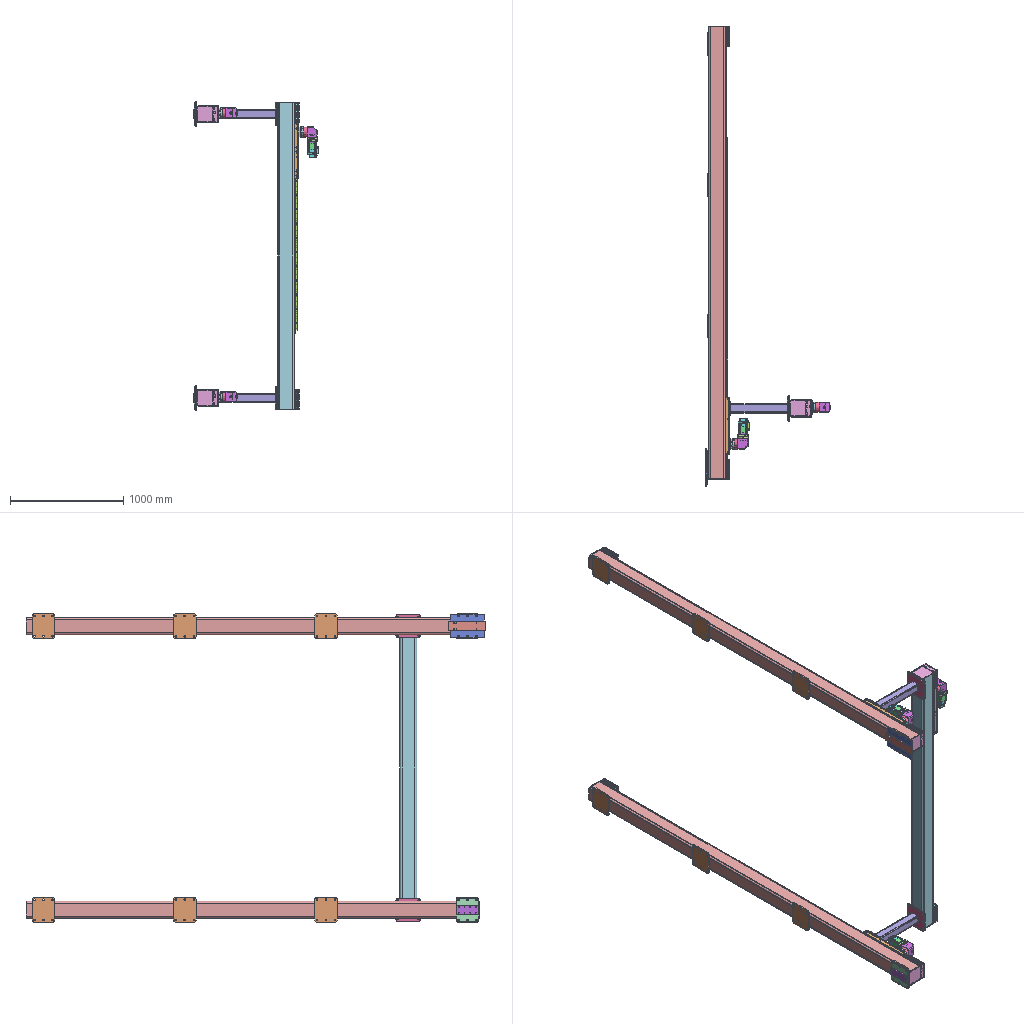Assembly | SolidWorks | 26 different items | 96 placed | box 1114 x 4070 x 2730 mm
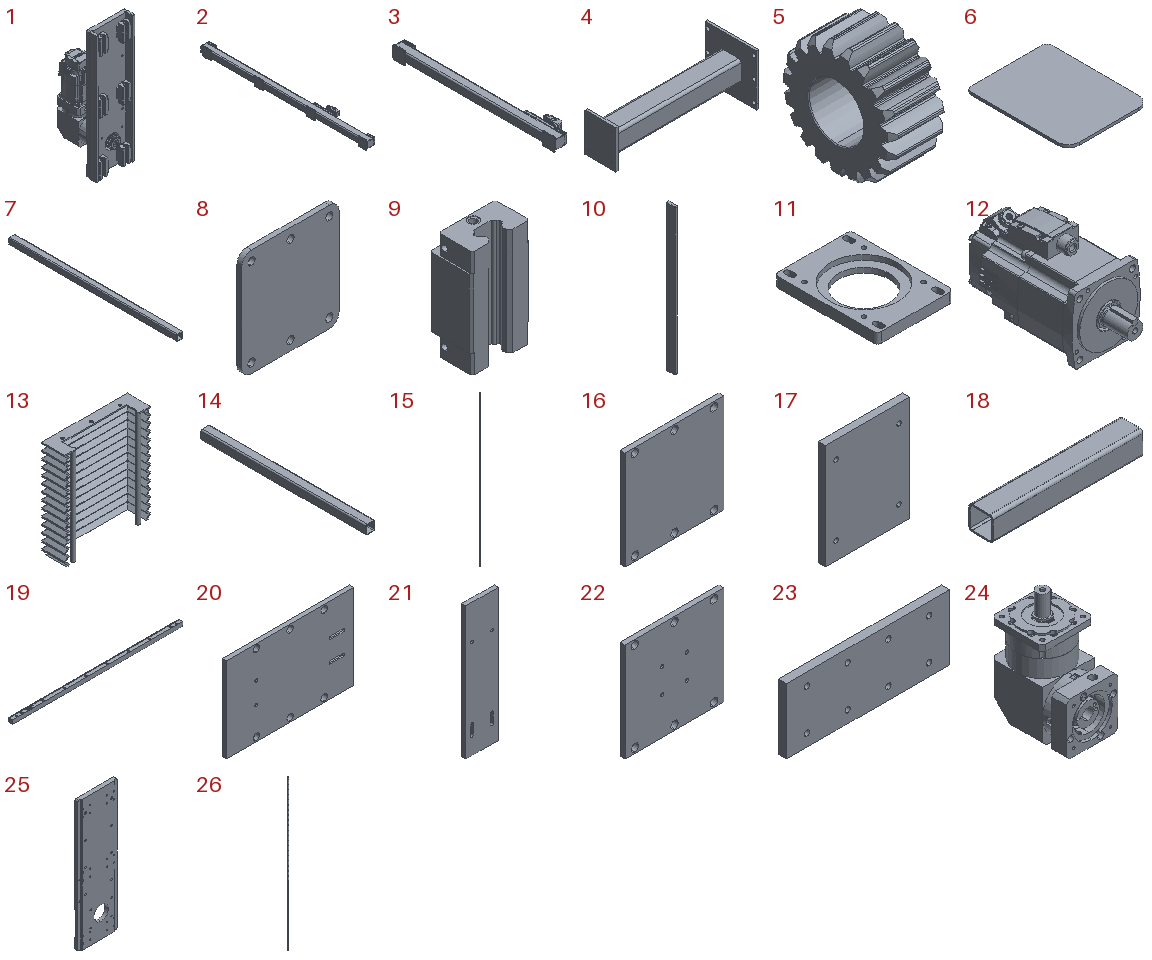Parts list (item | name | quantity | parent item | size | volume | features):
1 | (subassembly) | x3 | in 2, 3 | 150 x 216.98 x 500 mm | 3576400 mm3 | features ReferencePattern 5, LocalLPattern 1
2 | (subassembly) | x2 | - | - | 25579409 mm3 | features ReferencePattern 8, LocalLPattern 2, MirrorCompFeat 2
3 | (subassembly) | x1 | - | - | 18104640 mm3 | features ReferencePattern 5, LocalLPattern 2, MirrorCompFeat 2
4 | (subassembly) | x2 | - | 520 x 200 x 200 mm | 1285920 mm3 | -
5 | - | x3 | in 1 | 20 x 41.909 x 41.772 mm | 16148 mm3 | features MBimport 1
6 | - | x6 | in 2, 3 | 150 x 190 x 5 mm | 141427 mm3 | features Fillet 2, Extrusion 1
7 | - | x2 | in 2 | 150 x 4000 x 150 mm | 16889916 mm3 | features ICE 2, Extrusion 1, LPattern 1
8 | - | x10 | in 2, 3 | 200 x 10 x 220 mm | 425963 mm3 | features Extrusion 1, Fillet 1, ICE 1, LPattern 1
9 | - | x18 | in 1 | 34 x 23.7 x 61.4 mm | 36561 mm3 | features BaseBody 1
10 | - | x6 | in 1 | 8 x 29 x 500 mm | 115683 mm3 | features BaseBody 1
11 | - | x3 | in 1 | 90 x 122 x 12 mm | 79896 mm3 | features ICE 3, Extrusion 1, Fillet 1, HoleWzd 1
12 | - | x3 | in 1 | 82.337 x 174.253 x 100 mm | 739661 mm3 | features MBimport 1
13 | - | x6 | in 2, 3 | 149 x 40 x 170 mm | 114701 mm3 | features BaseBody 1, ICE 1
14 | - | x1 | in 3 | 150 x 2710 x 150 mm | 11443018 mm3 | features ICE 2, Extrusion 1, LPattern 1
15 | - | x4 | in 2 | 15 x 12.5 x 4000 mm | 674573 mm3 | features BaseBody 1
16 | - | x2 | in 4 | 200 x 10 x 200 mm | 389397 mm3 | features Extrusion 1, ICE 1, LPattern 1
17 | - | x2 | in 4 | 120 x 10 x 150 mm | 178713 mm3 | features Extrusion 1, ICE 1
18 | - | x2 | in 4 | 500 x 80 x 80 mm | 717810 mm3 | features WeldMemberFeat 1, WeldmentFeature 1
19 | - | x8 | in 2, 3 | 1005 x 24 x 24 mm | 516028 mm3 | features MBimport 1
20 | - | x1 | - | 300 x 10 x 200 mm | 580619 mm3 | features ICE 3, Extrusion 1, HoleWzd 1, LPattern 1
21 | - | x1 | - | 80 x 10 x 330 mm | 259332 mm3 | features Extrusion 1, HoleWzd 1, ICE 1
22 | - | x1 | - | 200 x 10 x 200 mm | 386374 mm3 | features Extrusion 1, HoleWzd 1, ICE 1, LPattern 1
23 | - | x1 | - | 200 x 10 x 80 mm | 157263 mm3 | features Extrusion 1, HoleWzd 1
24 | - | x3 | in 1 | 90 x 131.5 x 192.5 mm | 1289252 mm3 | features BaseBody 8
25 | - | x3 | in 1 | 150 x 15 x 500 mm | 1000700 mm3 | features BaseBody 1
26 | - | x2 | in 3 | 15 x 12.5 x 2043 mm | 344620 mm3 | features BaseBody 1, ICE 1
Mates (type | each side: item.copy, entity, surface, feature):
In the top assembly
Coincident | 6.1 face plane Boss-Extrude1 | 6.2 face plane Boss-Extrude1
Coincident | 8.1 face plane Boss-Extrude1 | 8.2 face plane Boss-Extrude1
Coincident | 25.1 face plane | 17.1 face plane Boss-Extrude1
Concentric | 25.1 face cylinder | 17.1 face cylinder Cut-Extrude1 | 2 times
Coincident | 25.2 face plane | 17.2 face plane Boss-Extrude1
Concentric | 25.2 face cylinder | 17.2 face cylinder Cut-Extrude1 | 2 times
Coincident | 16.1 face plane Boss-Extrude1 | 8.3 face plane Boss-Extrude1
Concentric | 16.2 face cylinder LPattern1 | 8.4 face cylinder LPattern1 | 2 times
Concentric | 16.1 face cylinder LPattern1 | 8.3 face cylinder Cut-Extrude1
Concentric | 16.1 face cylinder LPattern1 | 8.3 face cylinder LPattern1
Coincident | 8.1 face plane Boss-Extrude1 | 22.1 face plane Boss-Extrude1
Concentric | 8.1 face cylinder LPattern1 | 22.1 face cylinder LPattern1 | 2 times
Coincident | 23.1 face plane Boss-Extrude1 | 22.1 face plane Boss-Extrude1
Concentric | 23.1 face cylinder Ø6.6 (6.6) Diameter Hole1 | 22.1 face cylinder Hole Size (based on socket head cap screw type)1 | 2 times
Coincident | 8.2 face plane Boss-Extrude1 | 20.1 face plane Boss-Extrude1
Coincident | 8.2 edge | 20.1 face cylinder LPattern1
Concentric | 8.2 face cylinder LPattern1 | 20.1 face cylinder LPattern1
Coincident | 21.1 face plane Boss-Extrude1 | 20.1 face plane Boss-Extrude1
Concentric | 21.1 face cylinder Ø6.6 (6.6) Diameter Hole1 | 20.1 face cylinder Hole Size (based on socket head cap screw type)1 | 2 times
In subassembly 2
Coincident | 7.1 face plane Cut-Extrude1 | 19.1 face plane FXH Spur Rack SSFH[FXHSSFH021010].step | 2 times
Coincident | 7.1 face plane Boss-Extrude1 | 19.1 face plane FXH Spur Rack SSFH[FXHSSFH021010].step
Coincident | 7.1 face plane Boss-Extrude1 | 6.3 face plane Boss-Extrude1 | 3 times
Coincident | 15.1 face plane | 9.1 face plane DH150G-S3000-A2-T750W-C3.STEP-1/HGH15_23.STEP-6-solid1
Coincident | 7.1 face plane Boss-Extrude1 | 15.1 face plane
Coincident | 7.1 face plane Cut-Extrude1 | 15.1 face plane | 2 times
Width | 7.1 face plane Boss-Extrude1 | 7.1 face plane Boss-Extrude1 | 10.1 face plane | 10.2 face plane
LimitDistanceDim | 19.1 face plane FXH Spur Rack SSFH[FXHSSFH021010].step | 25.3 face plane
Coincident | 7.1 face plane Boss-Extrude1 | 13.1 face plane | 2 times
Coincident | 6.3 face plane Boss-Extrude1 | 13.1 face plane Cut-Extrude1
Coincident | 7.1 face plane Boss-Extrude1 | 8.5 face plane Boss-Extrude1
DistanceDim | 6.3 face plane Boss-Extrude1 | 8.5 face plane Boss-Extrude1
Width | 7.1 face plane Boss-Extrude1 | 7.1 face plane Boss-Extrude1 | 8.5 face plane Boss-Extrude1 | 8.5 face plane Boss-Extrude1
In subassembly 1
Coincident | 25.4 face plane | 10.3 face plane | 2 times
Coincident | 25.4 edge | 10.3 face plane
Concentric | 25.4 face cylinder | 9.2 face cylinder DH150G-S3000-A2-T750W-C3.STEP-1/HGH15_23.STEP-6-solid1 | 2 times
Coincident | 25.4 face plane | 9.2 face plane DH150G-S3000-A2-T750W-C3.STEP-1/HGH15_23.STEP-6-solid1
Coincident | 25.4 face plane | 10.4 face plane | 3 times
Coincident | 25.4 face plane | 11.1 face plane Boss-Extrude1 | 2 times
DistanceDim | 11.1 face plane Boss-Extrude1 | 25.4 face plane
Coincident | 11.1 face plane Boss-Extrude1 | 24.1 face plane
Concentric | 11.1 face cylinder M6 Tapped Hole1 | 24.1 face cylinder | 2 times
Coincident | 24.1 face plane | 12.1 face plane 1FL6042-2AF21-1AA1_3D_en.STP
Concentric | 24.1 face cylinder | 12.1 face cylinder 1FL6042-2AF21-1AA1_3D_en.STP
Parallel | 24.1 face cylinder | 12.1 face cylinder 1FL6042-2AF21-1AA1_3D_en.STP
Parallel | 24.1 face plane | 12.1 face plane 1FL6042-2AF21-1AA1_3D_en.STP
Concentric | 24.1 face cylinder | 5.1 face cylinder Standard Module 2 Spur Gear, 20&deg; Pressure Angle [GSEHC-2-19-20-dc20-A].step
DistanceDim | 24.1 face plane | 5.1 face plane Standard Module 2 Spur Gear, 20&deg; Pressure Angle [GSEHC-2-19-20-dc20-A].step
In subassembly 4
Coincident | 18.1 face plane Square Tube 80 X 80 X 5.0(1) | 17.3 face plane Boss-Extrude1
Width | 18.1 face plane Square Tube 80 X 80 X 5.0(1) | 18.1 face plane Square Tube 80 X 80 X 5.0(1) | 17.3 face plane Boss-Extrude1 | 17.3 face plane Boss-Extrude1
Width | 17.3 face plane Boss-Extrude1 | 17.3 face plane Boss-Extrude1 | 18.1 face plane Square Tube 80 X 80 X 5.0(1) | 18.1 face plane Square Tube 80 X 80 X 5.0(1)
Coincident | 18.1 face plane Square Tube 80 X 80 X 5.0(1) | 16.3 face plane Boss-Extrude1
Width | 18.1 face plane Square Tube 80 X 80 X 5.0(1) | 18.1 face plane Square Tube 80 X 80 X 5.0(1) | 16.3 face plane Boss-Extrude1 | 16.3 face plane Boss-Extrude1
Width | 16.3 face plane Boss-Extrude1 | 16.3 face plane Boss-Extrude1 | 18.1 face plane Square Tube 80 X 80 X 5.0(1) | 18.1 face plane Square Tube 80 X 80 X 5.0(1)
In subassembly 3
Coincident | 14.1 face plane Cut-Extrude1 | 19.1 face plane FXH Spur Rack SSFH[FXHSSFH021010].step | 2 times
Coincident | 14.1 face plane Boss-Extrude1 | 19.1 face plane FXH Spur Rack SSFH[FXHSSFH021010].step
Coincident | 14.1 face plane Boss-Extrude1 | 6.3 face plane Boss-Extrude1 | 3 times
Coincident | 26.1 face plane | 9.1 face plane DH150G-S3000-A2-T750W-C3.STEP-1/HGH15_23.STEP-6-solid1
Coincident | 14.1 face plane Boss-Extrude1 | 26.1 face plane
Coincident | 14.1 face plane Cut-Extrude1 | 26.1 face plane | 2 times
Width | 14.1 face plane Boss-Extrude1 | 14.1 face plane Boss-Extrude1 | 10.1 face plane | 10.2 face plane
LimitDistanceDim | 19.1 face plane FXH Spur Rack SSFH[FXHSSFH021010].step | 25.3 face plane
Coincident | 14.1 face plane Boss-Extrude1 | 13.1 face plane | 2 times
Coincident | 6.3 face plane Boss-Extrude1 | 13.1 face plane Cut-Extrude1
Coincident | 14.1 face plane Boss-Extrude1 | 8.5 face plane Boss-Extrude1
DistanceDim | 6.3 face plane Boss-Extrude1 | 8.5 face plane Boss-Extrude1
Width | 14.1 face plane Boss-Extrude1 | 14.1 face plane Boss-Extrude1 | 8.5 face plane Boss-Extrude1 | 8.5 face plane Boss-Extrude1